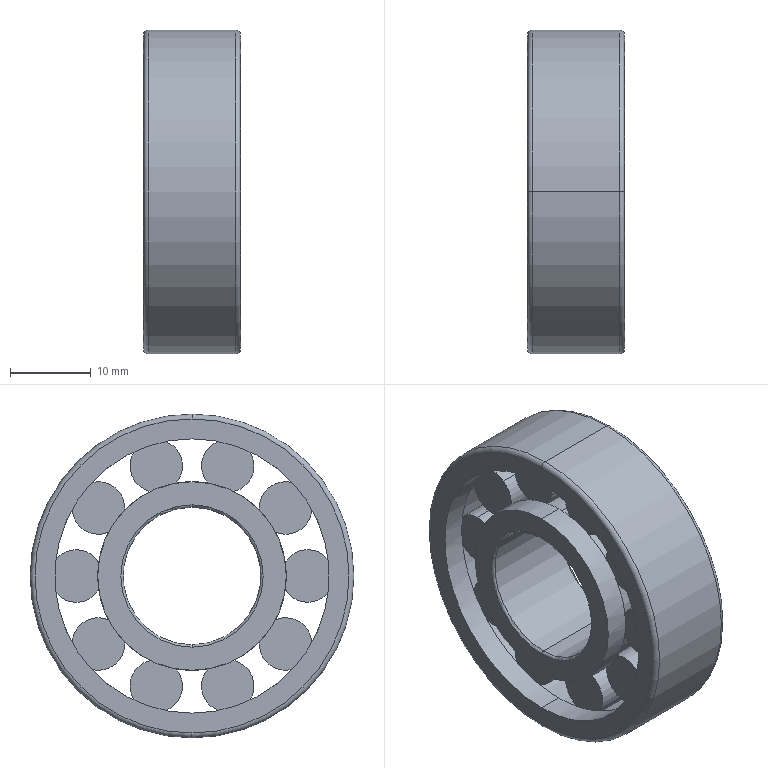Part | SolidWorks | features Revolution 3, CirPattern 1 | 1 solid | 136 faces | box 12 x 40 x 40 mm | volume 7964 mm3 | cylinder 64 | plane 64 | torus 8 | commonest cylinder face diameters 6.5 x30 22.1 x11 35.1 x11 23.3 x4 33.9 x4 17 x2